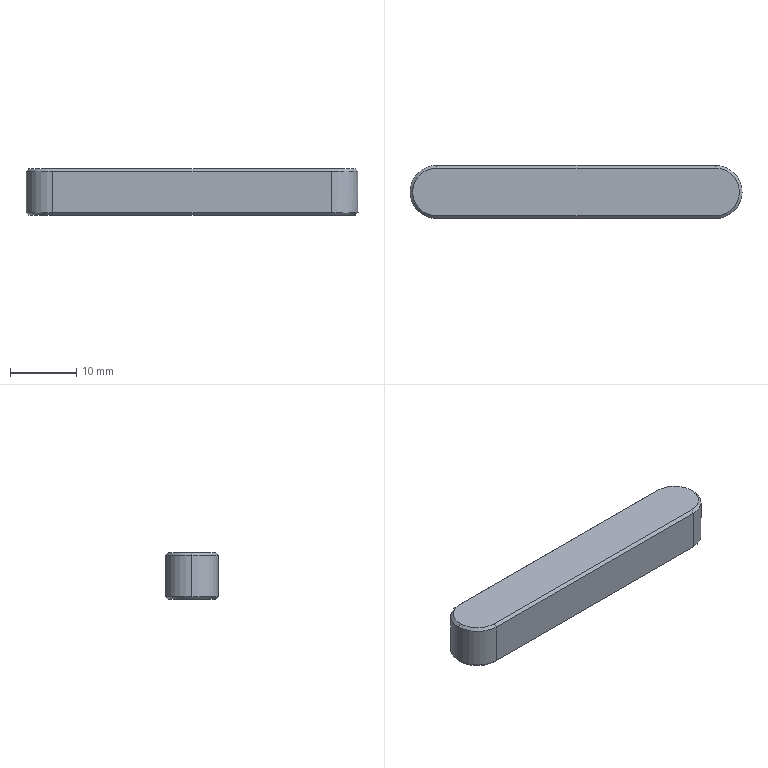Part | STEP file | plain parallel_keys_GB_CONNECTING_PIECE_KEYS_CSK 8X50 | 1 solid | 17 faces | box 50 x 8 x 7 mm | volume 2687 mm3 | plane 8 | cone 6 | cylinder 3 | commonest cylinder face diameters 8 x3
STEP:
#1=CARTESIAN_POINT('',(0.,0.,0.));
#2=DIRECTION('',(0.,0.,1.));
#3=DIRECTION('',(1.,0.,0.));
#4=AXIS2_PLACEMENT_3D('',#1,#2,#3);
#5=CARTESIAN_POINT('',(3.6,0.,-3.5));
#6=VERTEX_POINT('',#5);
#7=CARTESIAN_POINT('',(0.,-3.6,-3.5));
#8=VERTEX_POINT('',#7);
#9=CARTESIAN_POINT('',(0.,0.,-3.5));
#10=DIRECTION('',(0.,0.,-1.));
#11=DIRECTION('',(1.,0.,0.));
#12=AXIS2_PLACEMENT_3D('',#9,#10,#11);
#13=CIRCLE('',#12,3.6);
#14=CARTESIAN_POINT('',(0.,0.,-3.1));
#15=DIRECTION('',(0.,0.,1.));
#16=DIRECTION('',(1.,0.,0.));
#17=AXIS2_PLACEMENT_3D('',#14,#15,#16);
#18=CONICAL_SURFACE('',#17,4.,0.7854);
#19=CARTESIAN_POINT('',(6.283,-0.4));
#20=DIRECTION('',(-1.,0.));
#21=VECTOR('',#20,1.);
#22=LINE('',#19,#21);
#23=(GEOMETRIC_REPRESENTATION_CONTEXT(2)PARAMETRIC_REPRESENTATION_CONTEXT()REPRESENTATION_CONTEXT('',''));
#24=DEFINITIONAL_REPRESENTATION('',(#22),#23);
#25=PCURVE('',#18,#24);
#26=CARTESIAN_POINT('',(-42.,0.,-3.5));
#27=DIRECTION('',(0.,0.,-1.));
#28=DIRECTION('',(-1.,0.,0.));
#29=AXIS2_PLACEMENT_3D('',#26,#27,#28);
#30=PLANE('',#29);
#31=CARTESIAN_POINT('',(-42.,0.));
#32=DIRECTION('',(-1.,0.));
#33=AXIS2_PLACEMENT_2D('',#31,#32);
#34=CIRCLE('',#33,3.6);
#35=(GEOMETRIC_REPRESENTATION_CONTEXT(2)PARAMETRIC_REPRESENTATION_CONTEXT()REPRESENTATION_CONTEXT('',''));
#36=DEFINITIONAL_REPRESENTATION('',(#34),#35);
#37=PCURVE('',#30,#36);
#38=SURFACE_CURVE('',#13,(#25,#37),.PCURVE_S1.);
#39=EDGE_CURVE('',#6,#8,#38,.T.);
#40=ORIENTED_EDGE('',*,*,#39,.F.);
#41=CARTESIAN_POINT('',(4.,0.,-3.1));
#42=VERTEX_POINT('',#41);
#43=CARTESIAN_POINT('',(4.,0.,-3.1));
#44=DIRECTION('',(0.7071,0.,0.7071));
#45=VECTOR('',#44,1.);
#46=LINE('',#43,#45);
#47=CARTESIAN_POINT('',(6.283,0.));
#48=DIRECTION('',(0.,1.));
#49=VECTOR('',#48,1.);
#50=LINE('',#47,#49);
#51=(GEOMETRIC_REPRESENTATION_CONTEXT(2)PARAMETRIC_REPRESENTATION_CONTEXT()REPRESENTATION_CONTEXT('',''));
#52=DEFINITIONAL_REPRESENTATION('',(#50),#51);
#53=PCURVE('',#18,#52);
#54=CARTESIAN_POINT('',(0.,0.,-3.1));
#55=DIRECTION('',(0.,0.,1.));
#56=DIRECTION('',(1.,0.,0.));
#57=AXIS2_PLACEMENT_3D('',#54,#55,#56);
#58=CONICAL_SURFACE('',#57,4.,0.7854);
#59=CARTESIAN_POINT('',(0.,0.));
#60=DIRECTION('',(0.,1.));
#61=VECTOR('',#60,1.);
#62=LINE('',#59,#61);
#63=(GEOMETRIC_REPRESENTATION_CONTEXT(2)PARAMETRIC_REPRESENTATION_CONTEXT()REPRESENTATION_CONTEXT('',''));
#64=DEFINITIONAL_REPRESENTATION('',(#62),#63);
#65=PCURVE('',#58,#64);
#66=SURFACE_CURVE('',#46,(#53,#65),.PCURVE_S1.);
#67=EDGE_CURVE('',#6,#42,#66,.T.);
#68=ORIENTED_EDGE('',*,*,#67,.T.);
#69=CARTESIAN_POINT('',(0.,-4.,-3.1));
#70=VERTEX_POINT('',#69);
#71=CARTESIAN_POINT('',(0.,0.,-3.1));
#72=DIRECTION('',(0.,0.,-1.));
#73=DIRECTION('',(1.,0.,0.));
#74=AXIS2_PLACEMENT_3D('',#71,#72,#73);
#75=CIRCLE('',#74,4.);
#76=CARTESIAN_POINT('',(6.283,0.));
#77=DIRECTION('',(-1.,0.));
#78=VECTOR('',#77,1.);
#79=LINE('',#76,#78);
#80=(GEOMETRIC_REPRESENTATION_CONTEXT(2)PARAMETRIC_REPRESENTATION_CONTEXT()REPRESENTATION_CONTEXT('',''));
#81=DEFINITIONAL_REPRESENTATION('',(#79),#80);
#82=PCURVE('',#18,#81);
#83=CARTESIAN_POINT('',(0.,0.,3.5));
#84=DIRECTION('',(0.,0.,-1.));
#85=DIRECTION('',(-1.,0.,0.));
#86=AXIS2_PLACEMENT_3D('',#83,#84,#85);
#87=CYLINDRICAL_SURFACE('',#86,4.);
#88=CARTESIAN_POINT('',(3.142,6.6));
#89=DIRECTION('',(1.,0.));
#90=VECTOR('',#89,1.);
#91=LINE('',#88,#90);
#92=(GEOMETRIC_REPRESENTATION_CONTEXT(2)PARAMETRIC_REPRESENTATION_CONTEXT()REPRESENTATION_CONTEXT('',''));
#93=DEFINITIONAL_REPRESENTATION('',(#91),#92);
#94=PCURVE('',#87,#93);
#95=SURFACE_CURVE('',#75,(#82,#94),.PCURVE_S1.);
#96=EDGE_CURVE('',#42,#70,#95,.T.);
#97=ORIENTED_EDGE('',*,*,#96,.T.);
#98=CARTESIAN_POINT('',(0.,-4.,-3.1));
#99=DIRECTION('',(0.,-0.7071,0.7071));
#100=VECTOR('',#99,1.);
#101=LINE('',#98,#100);
#102=CARTESIAN_POINT('',(4.712,0.));
#103=DIRECTION('',(0.,1.));
#104=VECTOR('',#103,1.);
#105=LINE('',#102,#104);
#106=(GEOMETRIC_REPRESENTATION_CONTEXT(2)PARAMETRIC_REPRESENTATION_CONTEXT()REPRESENTATION_CONTEXT('',''));
#107=DEFINITIONAL_REPRESENTATION('',(#105),#106);
#108=PCURVE('',#18,#107);
#109=CARTESIAN_POINT('',(0.,-4.,-3.1));
#110=DIRECTION('',(0.,-0.7071,-0.7071));
#111=DIRECTION('',(0.,0.7071,-0.7071));
#112=AXIS2_PLACEMENT_3D('',#109,#110,#111);
#113=PLANE('',#112);
#114=CARTESIAN_POINT('',(0.,0.));
#115=DIRECTION('',(-1.,0.));
#116=VECTOR('',#115,1.);
#117=LINE('',#114,#116);
#118=(GEOMETRIC_REPRESENTATION_CONTEXT(2)PARAMETRIC_REPRESENTATION_CONTEXT()REPRESENTATION_CONTEXT('',''));
#119=DEFINITIONAL_REPRESENTATION('',(#117),#118);
#120=PCURVE('',#113,#119);
#121=SURFACE_CURVE('',#101,(#108,#120),.PCURVE_S1.);
#122=EDGE_CURVE('',#8,#70,#121,.T.);
#123=ORIENTED_EDGE('',*,*,#122,.F.);
#124=EDGE_LOOP('',(#40,#68,#97,#123));
#125=FACE_BOUND('',#124,.T.);
#126=ADVANCED_FACE('',(#125),#18,.T.);
#127=CARTESIAN_POINT('',(-42.,-4.,3.1));
#128=VERTEX_POINT('',#127);
#129=CARTESIAN_POINT('',(-46.,0.,3.1));
#130=VERTEX_POINT('',#129);
#131=CARTESIAN_POINT('',(-42.,0.,3.1));
#132=DIRECTION('',(0.,0.,-1.));
#133=DIRECTION('',(-1.,0.,0.));
#134=AXIS2_PLACEMENT_3D('',#131,#132,#133);
#135=CIRCLE('',#134,4.);
#136=CARTESIAN_POINT('',(-42.,0.,3.5));
#137=DIRECTION('',(0.,0.,-1.));
#138=DIRECTION('',(-1.,0.,0.));
#139=AXIS2_PLACEMENT_3D('',#136,#137,#138);
#140=CYLINDRICAL_SURFACE('',#139,4.);
#141=CARTESIAN_POINT('',(0.,0.4));
#142=DIRECTION('',(1.,0.));
#143=VECTOR('',#142,1.);
#144=LINE('',#141,#143);
#145=(GEOMETRIC_REPRESENTATION_CONTEXT(2)PARAMETRIC_REPRESENTATION_CONTEXT()REPRESENTATION_CONTEXT('',''));
#146=DEFINITIONAL_REPRESENTATION('',(#144),#145);
#147=PCURVE('',#140,#146);
#148=CARTESIAN_POINT('',(-42.,0.,3.1));
#149=DIRECTION('',(0.,0.,-1.));
#150=DIRECTION('',(-1.,0.,0.));
#151=AXIS2_PLACEMENT_3D('',#148,#149,#150);
#152=CONICAL_SURFACE('',#151,4.,0.7854);
#153=CARTESIAN_POINT('',(0.,0.));
#154=DIRECTION('',(1.,0.));
#155=VECTOR('',#154,1.);
#156=LINE('',#153,#155);
#157=(GEOMETRIC_REPRESENTATION_CONTEXT(2)PARAMETRIC_REPRESENTATION_CONTEXT()REPRESENTATION_CONTEXT('',''));
#158=DEFINITIONAL_REPRESENTATION('',(#156),#157);
#159=PCURVE('',#152,#158);
#160=SURFACE_CURVE('',#135,(#147,#159),.PCURVE_S1.);
#161=EDGE_CURVE('',#128,#130,#160,.T.);
#162=ORIENTED_EDGE('',*,*,#161,.T.);
#163=CARTESIAN_POINT('',(-46.,0.,-3.1));
#164=VERTEX_POINT('',#163);
#165=CARTESIAN_POINT('',(-46.,0.,3.5));
#166=DIRECTION('',(0.,0.,-1.));
#167=VECTOR('',#166,1.);
#168=LINE('',#165,#167);
#169=CARTESIAN_POINT('',(6.283,0.));
#170=DIRECTION('',(0.,1.));
#171=VECTOR('',#170,1.);
#172=LINE('',#169,#171);
#173=(GEOMETRIC_REPRESENTATION_CONTEXT(2)PARAMETRIC_REPRESENTATION_CONTEXT()REPRESENTATION_CONTEXT('',''));
#174=DEFINITIONAL_REPRESENTATION('',(#172),#173);
#175=PCURVE('',#140,#174);
#176=CARTESIAN_POINT('',(-42.,0.,3.5));
#177=DIRECTION('',(0.,0.,-1.));
#178=DIRECTION('',(-1.,0.,0.));
#179=AXIS2_PLACEMENT_3D('',#176,#177,#178);
#180=CYLINDRICAL_SURFACE('',#179,4.);
#181=CARTESIAN_POINT('',(0.,0.));
#182=DIRECTION('',(0.,1.));
#183=VECTOR('',#182,1.);
#184=LINE('',#181,#183);
#185=(GEOMETRIC_REPRESENTATION_CONTEXT(2)PARAMETRIC_REPRESENTATION_CONTEXT()REPRESENTATION_CONTEXT('',''));
#186=DEFINITIONAL_REPRESENTATION('',(#184),#185);
#187=PCURVE('',#180,#186);
#188=SURFACE_CURVE('',#168,(#175,#187),.PCURVE_S1.);
#189=EDGE_CURVE('',#130,#164,#188,.T.);
#190=ORIENTED_EDGE('',*,*,#189,.T.);
#191=CARTESIAN_POINT('',(-42.,-4.,-3.1));
#192=VERTEX_POINT('',#191);
#193=CARTESIAN_POINT('',(-42.,0.,-3.1));
#194=DIRECTION('',(0.,0.,-1.));
#195=DIRECTION('',(1.,0.,0.));
#196=AXIS2_PLACEMENT_3D('',#193,#194,#195);
#197=CIRCLE('',#196,4.);
#198=CARTESIAN_POINT('',(3.142,6.6));
#199=DIRECTION('',(1.,0.));
#200=VECTOR('',#199,1.);
#201=LINE('',#198,#200);
#202=(GEOMETRIC_REPRESENTATION_CONTEXT(2)PARAMETRIC_REPRESENTATION_CONTEXT()REPRESENTATION_CONTEXT('',''));
#203=DEFINITIONAL_REPRESENTATION('',(#201),#202);
#204=PCURVE('',#140,#203);
#205=CARTESIAN_POINT('',(-42.,0.,-3.1));
#206=DIRECTION('',(0.,0.,1.));
#207=DIRECTION('',(1.,0.,0.));
#208=AXIS2_PLACEMENT_3D('',#205,#206,#207);
#209=CONICAL_SURFACE('',#208,4.,0.7854);
#210=CARTESIAN_POINT('',(6.283,0.));
#211=DIRECTION('',(-1.,0.));
#212=VECTOR('',#211,1.);
#213=LINE('',#210,#212);
#214=(GEOMETRIC_REPRESENTATION_CONTEXT(2)PARAMETRIC_REPRESENTATION_CONTEXT()REPRESENTATION_CONTEXT('',''));
#215=DEFINITIONAL_REPRESENTATION('',(#213),#214);
#216=PCURVE('',#209,#215);
#217=SURFACE_CURVE('',#197,(#204,#216),.PCURVE_S1.);
#218=EDGE_CURVE('',#192,#164,#217,.T.);
#219=ORIENTED_EDGE('',*,*,#218,.F.);
#220=CARTESIAN_POINT('',(-42.,-4.,3.5));
#221=DIRECTION('',(0.,0.,1.));
#222=VECTOR('',#221,1.);
#223=LINE('',#220,#222);
#224=CARTESIAN_POINT('',(4.712,0.));
#225=DIRECTION('',(0.,-1.));
#226=VECTOR('',#225,1.);
#227=LINE('',#224,#226);
#228=(GEOMETRIC_REPRESENTATION_CONTEXT(2)PARAMETRIC_REPRESENTATION_CONTEXT()REPRESENTATION_CONTEXT('',''));
#229=DEFINITIONAL_REPRESENTATION('',(#227),#228);
#230=PCURVE('',#140,#229);
#231=CARTESIAN_POINT('',(0.,-4.,3.5));
#232=DIRECTION('',(0.,1.,0.));
#233=DIRECTION('',(-1.,0.,0.));
#234=AXIS2_PLACEMENT_3D('',#231,#232,#233);
#235=PLANE('',#234);
#236=CARTESIAN_POINT('',(42.,0.));
#237=DIRECTION('',(0.,1.));
#238=VECTOR('',#237,1.);
#239=LINE('',#236,#238);
#240=(GEOMETRIC_REPRESENTATION_CONTEXT(2)PARAMETRIC_REPRESENTATION_CONTEXT()REPRESENTATION_CONTEXT('',''));
#241=DEFINITIONAL_REPRESENTATION('',(#239),#240);
#242=PCURVE('',#235,#241);
#243=SURFACE_CURVE('',#223,(#230,#242),.PCURVE_S1.);
#244=EDGE_CURVE('',#192,#128,#243,.T.);
#245=ORIENTED_EDGE('',*,*,#244,.T.);
#246=EDGE_LOOP('',(#162,#190,#219,#245));
#247=FACE_BOUND('',#246,.T.);
#248=ADVANCED_FACE('',(#247),#140,.T.);
#249=CARTESIAN_POINT('',(-42.,-3.6,3.5));
#250=VERTEX_POINT('',#249);
#251=CARTESIAN_POINT('',(-45.6,0.,3.5));
#252=VERTEX_POINT('',#251);
#253=CARTESIAN_POINT('',(-42.,0.,3.5));
#254=DIRECTION('',(0.,0.,-1.));
#255=DIRECTION('',(-1.,0.,0.));
#256=AXIS2_PLACEMENT_3D('',#253,#254,#255);
#257=CIRCLE('',#256,3.6);
#258=CARTESIAN_POINT('',(0.,-0.4));
#259=DIRECTION('',(1.,0.));
#260=VECTOR('',#259,1.);
#261=LINE('',#258,#260);
#262=(GEOMETRIC_REPRESENTATION_CONTEXT(2)PARAMETRIC_REPRESENTATION_CONTEXT()REPRESENTATION_CONTEXT('',''));
#263=DEFINITIONAL_REPRESENTATION('',(#261),#262);
#264=PCURVE('',#152,#263);
#265=CARTESIAN_POINT('',(-42.,0.,3.5));
#266=DIRECTION('',(0.,0.,-1.));
#267=DIRECTION('',(-1.,0.,0.));
#268=AXIS2_PLACEMENT_3D('',#265,#266,#267);
#269=PLANE('',#268);
#270=CARTESIAN_POINT('',(0.,0.));
#271=DIRECTION('',(1.,0.));
#272=AXIS2_PLACEMENT_2D('',#270,#271);
#273=CIRCLE('',#272,3.6);
#274=(GEOMETRIC_REPRESENTATION_CONTEXT(2)PARAMETRIC_REPRESENTATION_CONTEXT()REPRESENTATION_CONTEXT('',''));
#275=DEFINITIONAL_REPRESENTATION('',(#273),#274);
#276=PCURVE('',#269,#275);
#277=SURFACE_CURVE('',#257,(#264,#276),.PCURVE_S1.);
#278=EDGE_CURVE('',#250,#252,#277,.T.);
#279=ORIENTED_EDGE('',*,*,#278,.T.);
#280=CARTESIAN_POINT('',(-46.,0.,3.1));
#281=DIRECTION('',(-0.7071,0.,-0.7071));
#282=VECTOR('',#281,1.);
#283=LINE('',#280,#282);
#284=CARTESIAN_POINT('',(6.283,0.));
#285=DIRECTION('',(0.,1.));
#286=VECTOR('',#285,1.);
#287=LINE('',#284,#286);
#288=(GEOMETRIC_REPRESENTATION_CONTEXT(2)PARAMETRIC_REPRESENTATION_CONTEXT()REPRESENTATION_CONTEXT('',''));
#289=DEFINITIONAL_REPRESENTATION('',(#287),#288);
#290=PCURVE('',#152,#289);
#291=CARTESIAN_POINT('',(-42.,0.,3.1));
#292=DIRECTION('',(0.,0.,-1.));
#293=DIRECTION('',(-1.,0.,0.));
#294=AXIS2_PLACEMENT_3D('',#291,#292,#293);
#295=CONICAL_SURFACE('',#294,4.,0.7854);
#296=CARTESIAN_POINT('',(0.,0.));
#297=DIRECTION('',(0.,1.));
#298=VECTOR('',#297,1.);
#299=LINE('',#296,#298);
#300=(GEOMETRIC_REPRESENTATION_CONTEXT(2)PARAMETRIC_REPRESENTATION_CONTEXT()REPRESENTATION_CONTEXT('',''));
#301=DEFINITIONAL_REPRESENTATION('',(#299),#300);
#302=PCURVE('',#295,#301);
#303=SURFACE_CURVE('',#283,(#290,#302),.PCURVE_S1.);
#304=EDGE_CURVE('',#252,#130,#303,.T.);
#305=ORIENTED_EDGE('',*,*,#304,.T.);
#306=ORIENTED_EDGE('',*,*,#161,.F.);
#307=CARTESIAN_POINT('',(-42.,-498958.,-498950.9));
#308=DIRECTION('',(0.,0.7071,0.7071));
#309=VECTOR('',#308,1.);
#310=LINE('',#307,#309);
#311=CARTESIAN_POINT('',(4.712,498954.));
#312=DIRECTION('',(0.,-1.));
#313=VECTOR('',#312,1.);
#314=LINE('',#311,#313);
#315=(GEOMETRIC_REPRESENTATION_CONTEXT(2)PARAMETRIC_REPRESENTATION_CONTEXT()REPRESENTATION_CONTEXT('',''));
#316=DEFINITIONAL_REPRESENTATION('',(#314),#315);
#317=PCURVE('',#152,#316);
#318=CARTESIAN_POINT('',(-42.,-3.6,3.5));
#319=DIRECTION('',(0.,0.7071,-0.7071));
#320=DIRECTION('',(0.,0.7071,0.7071));
#321=AXIS2_PLACEMENT_3D('',#318,#319,#320);
#322=PLANE('',#321);
#323=CARTESIAN_POINT('',(-705628.079,0.));
#324=DIRECTION('',(1.,0.));
#325=VECTOR('',#324,1.);
#326=LINE('',#323,#325);
#327=(GEOMETRIC_REPRESENTATION_CONTEXT(2)PARAMETRIC_REPRESENTATION_CONTEXT()REPRESENTATION_CONTEXT('',''));
#328=DEFINITIONAL_REPRESENTATION('',(#326),#327);
#329=PCURVE('',#322,#328);
#330=SURFACE_CURVE('',#310,(#317,#329),.PCURVE_S1.);
#331=EDGE_CURVE('',#128,#250,#330,.T.);
#332=ORIENTED_EDGE('',*,*,#331,.T.);
#333=EDGE_LOOP('',(#279,#305,#306,#332));
#334=FACE_BOUND('',#333,.T.);
#335=ADVANCED_FACE('',(#334),#152,.T.);
#336=CARTESIAN_POINT('',(-42.,-3.6,-3.5));
#337=VERTEX_POINT('',#336);
#338=CARTESIAN_POINT('',(-42.,3.6,-3.5));
#339=VERTEX_POINT('',#338);
#340=CARTESIAN_POINT('',(-42.,0.,-3.5));
#341=DIRECTION('',(0.,0.,-1.));
#342=DIRECTION('',(1.,0.,0.));
#343=AXIS2_PLACEMENT_3D('',#340,#341,#342);
#344=CIRCLE('',#343,3.6);
#345=CARTESIAN_POINT('',(0.,0.));
#346=DIRECTION('',(-1.,0.));
#347=AXIS2_PLACEMENT_2D('',#345,#346);
#348=CIRCLE('',#347,3.6);
#349=(GEOMETRIC_REPRESENTATION_CONTEXT(2)PARAMETRIC_REPRESENTATION_CONTEXT()REPRESENTATION_CONTEXT('',''));
#350=DEFINITIONAL_REPRESENTATION('',(#348),#349);
#351=PCURVE('',#30,#350);
#352=CARTESIAN_POINT('',(6.283,-0.4));
#353=DIRECTION('',(-1.,0.));
#354=VECTOR('',#353,1.);
#355=LINE('',#352,#354);
#356=(GEOMETRIC_REPRESENTATION_CONTEXT(2)PARAMETRIC_REPRESENTATION_CONTEXT()REPRESENTATION_CONTEXT('',''));
#357=DEFINITIONAL_REPRESENTATION('',(#355),#356);
#358=PCURVE('',#209,#357);
#359=SURFACE_CURVE('',#344,(#351,#358),.PCURVE_S1.);
#360=EDGE_CURVE('',#337,#339,#359,.T.);
#361=ORIENTED_EDGE('',*,*,#360,.T.);
#362=CARTESIAN_POINT('',(0.,3.6,-3.5));
#363=VERTEX_POINT('',#362);
#364=CARTESIAN_POINT('',(-42.,3.6,-3.5));
#365=DIRECTION('',(1.,0.,0.));
#366=VECTOR('',#365,1.);
#367=LINE('',#364,#366);
#368=CARTESIAN_POINT('',(0.,3.6));
#369=DIRECTION('',(-1.,0.));
#370=VECTOR('',#369,1.);
#371=LINE('',#368,#370);
#372=(GEOMETRIC_REPRESENTATION_CONTEXT(2)PARAMETRIC_REPRESENTATION_CONTEXT()REPRESENTATION_CONTEXT('',''));
#373=DEFINITIONAL_REPRESENTATION('',(#371),#372);
#374=PCURVE('',#30,#373);
#375=CARTESIAN_POINT('',(-42.,4.,-3.1));
#376=DIRECTION('',(0.,0.7071,-0.7071));
#377=DIRECTION('',(0.,0.7071,0.7071));
#378=AXIS2_PLACEMENT_3D('',#375,#376,#377);
#379=PLANE('',#378);
#380=CARTESIAN_POINT('',(-0.5657,0.));
#381=DIRECTION('',(0.,1.));
#382=VECTOR('',#381,1.);
#383=LINE('',#380,#382);
#384=(GEOMETRIC_REPRESENTATION_CONTEXT(2)PARAMETRIC_REPRESENTATION_CONTEXT()REPRESENTATION_CONTEXT('',''));
#385=DEFINITIONAL_REPRESENTATION('',(#383),#384);
#386=PCURVE('',#379,#385);
#387=SURFACE_CURVE('',#367,(#374,#386),.PCURVE_S1.);
#388=EDGE_CURVE('',#339,#363,#387,.T.);
#389=ORIENTED_EDGE('',*,*,#388,.T.);
#390=CARTESIAN_POINT('',(0.,0.,-3.5));
#391=DIRECTION('',(0.,0.,-1.));
#392=DIRECTION('',(1.,0.,0.));
#393=AXIS2_PLACEMENT_3D('',#390,#391,#392);
#394=CIRCLE('',#393,3.6);
#395=CARTESIAN_POINT('',(-42.,0.));
#396=DIRECTION('',(-1.,0.));
#397=AXIS2_PLACEMENT_2D('',#395,#396);
#398=CIRCLE('',#397,3.6);
#399=(GEOMETRIC_REPRESENTATION_CONTEXT(2)PARAMETRIC_REPRESENTATION_CONTEXT()REPRESENTATION_CONTEXT('',''));
#400=DEFINITIONAL_REPRESENTATION('',(#398),#399);
#401=PCURVE('',#30,#400);
#402=CARTESIAN_POINT('',(6.283,-0.4));
#403=DIRECTION('',(-1.,0.));
#404=VECTOR('',#403,1.);
#405=LINE('',#402,#404);
#406=(GEOMETRIC_REPRESENTATION_CONTEXT(2)PARAMETRIC_REPRESENTATION_CONTEXT()REPRESENTATION_CONTEXT('',''));
#407=DEFINITIONAL_REPRESENTATION('',(#405),#406);
#408=PCURVE('',#58,#407);
#409=SURFACE_CURVE('',#394,(#401,#408),.PCURVE_S1.);
#410=EDGE_CURVE('',#363,#6,#409,.T.);
#411=ORIENTED_EDGE('',*,*,#410,.T.);
#412=ORIENTED_EDGE('',*,*,#39,.T.);
#413=CARTESIAN_POINT('',(-42.,-3.6,-3.5));
#414=DIRECTION('',(-1.,0.,0.));
#415=VECTOR('',#414,1.);
#416=LINE('',#413,#415);
#417=CARTESIAN_POINT('',(0.,-3.6));
#418=DIRECTION('',(1.,0.));
#419=VECTOR('',#418,1.);
#420=LINE('',#417,#419);
#421=(GEOMETRIC_REPRESENTATION_CONTEXT(2)PARAMETRIC_REPRESENTATION_CONTEXT()REPRESENTATION_CONTEXT('',''));
#422=DEFINITIONAL_REPRESENTATION('',(#420),#421);
#423=PCURVE('',#30,#422);
#424=CARTESIAN_POINT('',(0.5657,-42.));
#425=DIRECTION('',(0.,-1.));
#426=VECTOR('',#425,1.);
#427=LINE('',#424,#426);
#428=(GEOMETRIC_REPRESENTATION_CONTEXT(2)PARAMETRIC_REPRESENTATION_CONTEXT()REPRESENTATION_CONTEXT('',''));
#429=DEFINITIONAL_REPRESENTATION('',(#427),#428);
#430=PCURVE('',#113,#429);
#431=SURFACE_CURVE('',#416,(#423,#430),.PCURVE_S1.);
#432=EDGE_CURVE('',#8,#337,#431,.T.);
#433=ORIENTED_EDGE('',*,*,#432,.T.);
#434=EDGE_LOOP('',(#361,#389,#411,#412,#433));
#435=FACE_BOUND('',#434,.T.);
#436=ADVANCED_FACE('',(#435),#30,.T.);
#437=CARTESIAN_POINT('',(-42.,4.,-3.1));
#438=VERTEX_POINT('',#437);
#439=CARTESIAN_POINT('',(-42.,4.,-3.1));
#440=DIRECTION('',(0.,0.7071,0.7071));
#441=VECTOR('',#440,1.);
#442=LINE('',#439,#441);
#443=CARTESIAN_POINT('',(0.,0.));
#444=DIRECTION('',(1.,0.));
#445=VECTOR('',#444,1.);
#446=LINE('',#443,#445);
#447=(GEOMETRIC_REPRESENTATION_CONTEXT(2)PARAMETRIC_REPRESENTATION_CONTEXT()REPRESENTATION_CONTEXT('',''));
#448=DEFINITIONAL_REPRESENTATION('',(#446),#447);
#449=PCURVE('',#379,#448);
#450=CARTESIAN_POINT('',(1.571,0.));
#451=DIRECTION('',(0.,1.));
#452=VECTOR('',#451,1.);
#453=LINE('',#450,#452);
#454=(GEOMETRIC_REPRESENTATION_CONTEXT(2)PARAMETRIC_REPRESENTATION_CONTEXT()REPRESENTATION_CONTEXT('',''));
#455=DEFINITIONAL_REPRESENTATION('',(#453),#454);
#456=PCURVE('',#209,#455);
#457=SURFACE_CURVE('',#442,(#449,#456),.PCURVE_S1.);
#458=EDGE_CURVE('',#339,#438,#457,.T.);
#459=ORIENTED_EDGE('',*,*,#458,.T.);
#460=CARTESIAN_POINT('',(0.,4.,-3.1));
#461=VERTEX_POINT('',#460);
#462=CARTESIAN_POINT('',(-42.,4.,-3.1));
#463=DIRECTION('',(1.,0.,0.));
#464=VECTOR('',#463,1.);
#465=LINE('',#462,#464);
#466=CARTESIAN_POINT('',(0.,0.));
#467=DIRECTION('',(0.,1.));
#468=VECTOR('',#467,1.);
#469=LINE('',#466,#468);
#470=(GEOMETRIC_REPRESENTATION_CONTEXT(2)PARAMETRIC_REPRESENTATION_CONTEXT()REPRESENTATION_CONTEXT('',''));
#471=DEFINITIONAL_REPRESENTATION('',(#469),#470);
#472=PCURVE('',#379,#471);
#473=CARTESIAN_POINT('',(-42.,4.,3.5));
#474=DIRECTION('',(0.,-1.,0.));
#475=DIRECTION('',(1.,0.,0.));
#476=AXIS2_PLACEMENT_3D('',#473,#474,#475);
#477=PLANE('',#476);
#478=CARTESIAN_POINT('',(0.,-6.6));
#479=DIRECTION('',(1.,0.));
#480=VECTOR('',#479,1.);
#481=LINE('',#478,#480);
#482=(GEOMETRIC_REPRESENTATION_CONTEXT(2)PARAMETRIC_REPRESENTATION_CONTEXT()REPRESENTATION_CONTEXT('',''));
#483=DEFINITIONAL_REPRESENTATION('',(#481),#482);
#484=PCURVE('',#477,#483);
#485=SURFACE_CURVE('',#465,(#472,#484),.PCURVE_S1.);
#486=EDGE_CURVE('',#438,#461,#485,.T.);
#487=ORIENTED_EDGE('',*,*,#486,.T.);
#488=CARTESIAN_POINT('',(0.,4.,-3.1));
#489=DIRECTION('',(0.,-0.7071,-0.7071));
#490=VECTOR('',#489,1.);
#491=LINE('',#488,#490);
#492=CARTESIAN_POINT('',(0.,42.));
#493=DIRECTION('',(-1.,0.));
#494=VECTOR('',#493,1.);
#495=LINE('',#492,#494);
#496=(GEOMETRIC_REPRESENTATION_CONTEXT(2)PARAMETRIC_REPRESENTATION_CONTEXT()REPRESENTATION_CONTEXT('',''));
#497=DEFINITIONAL_REPRESENTATION('',(#495),#496);
#498=PCURVE('',#379,#497);
#499=CARTESIAN_POINT('',(1.571,0.));
#500=DIRECTION('',(0.,-1.));
#501=VECTOR('',#500,1.);
#502=LINE('',#499,#501);
#503=(GEOMETRIC_REPRESENTATION_CONTEXT(2)PARAMETRIC_REPRESENTATION_CONTEXT()REPRESENTATION_CONTEXT('',''));
#504=DEFINITIONAL_REPRESENTATION('',(#502),#503);
#505=PCURVE('',#58,#504);
#506=SURFACE_CURVE('',#491,(#498,#505),.PCURVE_S1.);
#507=EDGE_CURVE('',#461,#363,#506,.T.);
#508=ORIENTED_EDGE('',*,*,#507,.T.);
#509=ORIENTED_EDGE('',*,*,#388,.F.);
#510=EDGE_LOOP('',(#459,#487,#508,#509));
#511=FACE_BOUND('',#510,.T.);
#512=ADVANCED_FACE('',(#511),#379,.T.);
#513=CARTESIAN_POINT('',(-42.,-499007.1,499000.));
#514=DIRECTION('',(0.,-0.7071,0.7071));
#515=VECTOR('',#514,1.);
#516=LINE('',#513,#515);
#517=CARTESIAN_POINT('',(4.712,499003.1));
#518=DIRECTION('',(0.,1.));
#519=VECTOR('',#518,1.);
#520=LINE('',#517,#519);
#521=(GEOMETRIC_REPRESENTATION_CONTEXT(2)PARAMETRIC_REPRESENTATION_CONTEXT()REPRESENTATION_CONTEXT('',''));
#522=DEFINITIONAL_REPRESENTATION('',(#520),#521);
#523=PCURVE('',#209,#522);
#524=CARTESIAN_POINT('',(-705696.952,-42.));
#525=DIRECTION('',(-1.,0.));
#526=VECTOR('',#525,1.);
#527=LINE('',#524,#526);
#528=(GEOMETRIC_REPRESENTATION_CONTEXT(2)PARAMETRIC_REPRESENTATION_CONTEXT()REPRESENTATION_CONTEXT('',''));
#529=DEFINITIONAL_REPRESENTATION('',(#527),#528);
#530=PCURVE('',#113,#529);
#531=SURFACE_CURVE('',#516,(#523,#530),.PCURVE_S1.);
#532=EDGE_CURVE('',#337,#192,#531,.T.);
#533=ORIENTED_EDGE('',*,*,#532,.T.);
#534=ORIENTED_EDGE('',*,*,#218,.T.);
#535=CARTESIAN_POINT('',(-42.,0.,-3.1));
#536=DIRECTION('',(0.,0.,-1.));
#537=DIRECTION('',(1.,0.,0.));
#538=AXIS2_PLACEMENT_3D('',#535,#536,#537);
#539=CIRCLE('',#538,4.);
#540=CARTESIAN_POINT('',(6.283,0.));
#541=DIRECTION('',(-1.,0.));
#542=VECTOR('',#541,1.);
#543=LINE('',#540,#542);
#544=(GEOMETRIC_REPRESENTATION_CONTEXT(2)PARAMETRIC_REPRESENTATION_CONTEXT()REPRESENTATION_CONTEXT('',''));
#545=DEFINITIONAL_REPRESENTATION('',(#543),#544);
#546=PCURVE('',#209,#545);
#547=CARTESIAN_POINT('',(-3.142,6.6));
#548=DIRECTION('',(1.,0.));
#549=VECTOR('',#548,1.);
#550=LINE('',#547,#549);
#551=(GEOMETRIC_REPRESENTATION_CONTEXT(2)PARAMETRIC_REPRESENTATION_CONTEXT()REPRESENTATION_CONTEXT('',''));
#552=DEFINITIONAL_REPRESENTATION('',(#550),#551);
#553=PCURVE('',#180,#552);
#554=SURFACE_CURVE('',#539,(#546,#553),.PCURVE_S1.);
#555=EDGE_CURVE('',#164,#438,#554,.T.);
#556=ORIENTED_EDGE('',*,*,#555,.T.);
#557=ORIENTED_EDGE('',*,*,#458,.F.);
#558=ORIENTED_EDGE('',*,*,#360,.F.);
#559=EDGE_LOOP('',(#533,#534,#556,#557,#558));
#560=FACE_BOUND('',#559,.T.);
#561=ADVANCED_FACE('',(#560),#209,.T.);
#562=ORIENTED_EDGE('',*,*,#122,.T.);
#563=CARTESIAN_POINT('',(0.,-4.,-3.1));
#564=DIRECTION('',(-1.,0.,0.));
#565=VECTOR('',#564,1.);
#566=LINE('',#563,#565);
#567=CARTESIAN_POINT('',(0.,0.));
#568=DIRECTION('',(0.,-1.));
#569=VECTOR('',#568,1.);
#570=LINE('',#567,#569);
#571=(GEOMETRIC_REPRESENTATION_CONTEXT(2)PARAMETRIC_REPRESENTATION_CONTEXT()REPRESENTATION_CONTEXT('',''));
#572=DEFINITIONAL_REPRESENTATION('',(#570),#571);
#573=PCURVE('',#113,#572);
#574=CARTESIAN_POINT('',(0.,-6.6));
#575=DIRECTION('',(1.,0.));
#576=VECTOR('',#575,1.);
#577=LINE('',#574,#576);
#578=(GEOMETRIC_REPRESENTATION_CONTEXT(2)PARAMETRIC_REPRESENTATION_CONTEXT()REPRESENTATION_CONTEXT('',''));
#579=DEFINITIONAL_REPRESENTATION('',(#577),#578);
#580=PCURVE('',#235,#579);
#581=SURFACE_CURVE('',#566,(#573,#580),.PCURVE_S1.);
#582=EDGE_CURVE('',#70,#192,#581,.T.);
#583=ORIENTED_EDGE('',*,*,#582,.T.);
#584=ORIENTED_EDGE('',*,*,#532,.F.);
#585=ORIENTED_EDGE('',*,*,#432,.F.);
#586=EDGE_LOOP('',(#562,#583,#584,#585));
#587=FACE_BOUND('',#586,.T.);
#588=ADVANCED_FACE('',(#587),#113,.T.);
#589=ORIENTED_EDGE('',*,*,#67,.F.);
#590=ORIENTED_EDGE('',*,*,#410,.F.);
#591=ORIENTED_EDGE('',*,*,#507,.F.);
#592=CARTESIAN_POINT('',(0.,0.,-3.1));
#593=DIRECTION('',(0.,0.,-1.));
#594=DIRECTION('',(1.,0.,0.));
#595=AXIS2_PLACEMENT_3D('',#592,#593,#594);
#596=CIRCLE('',#595,4.);
#597=CARTESIAN_POINT('',(6.283,0.));
#598=DIRECTION('',(-1.,0.));
#599=VECTOR('',#598,1.);
#600=LINE('',#597,#599);
#601=(GEOMETRIC_REPRESENTATION_CONTEXT(2)PARAMETRIC_REPRESENTATION_CONTEXT()REPRESENTATION_CONTEXT('',''));
#602=DEFINITIONAL_REPRESENTATION('',(#600),#601);
#603=PCURVE('',#58,#602);
#604=CARTESIAN_POINT('',(-3.142,6.6));
#605=DIRECTION('',(1.,0.));
#606=VECTOR('',#605,1.);
#607=LINE('',#604,#606);
#608=(GEOMETRIC_REPRESENTATION_CONTEXT(2)PARAMETRIC_REPRESENTATION_CONTEXT()REPRESENTATION_CONTEXT('',''));
#609=DEFINITIONAL_REPRESENTATION('',(#607),#608);
#610=PCURVE('',#87,#609);
#611=SURFACE_CURVE('',#596,(#603,#610),.PCURVE_S1.);
#612=EDGE_CURVE('',#461,#42,#611,.T.);
#613=ORIENTED_EDGE('',*,*,#612,.T.);
#614=EDGE_LOOP('',(#589,#590,#591,#613));
#615=FACE_BOUND('',#614,.T.);
#616=ADVANCED_FACE('',(#615),#58,.T.);
#617=CARTESIAN_POINT('',(0.,4.,3.1));
#618=VERTEX_POINT('',#617);
#619=CARTESIAN_POINT('',(-42.,4.,3.1));
#620=VERTEX_POINT('',#619);
#621=CARTESIAN_POINT('',(-42.,4.,3.1));
#622=DIRECTION('',(-1.,0.,0.));
#623=VECTOR('',#622,1.);
#624=LINE('',#621,#623);
#625=CARTESIAN_POINT('',(0.,-0.4));
#626=DIRECTION('',(-1.,0.));
#627=VECTOR('',#626,1.);
#628=LINE('',#625,#627);
#629=(GEOMETRIC_REPRESENTATION_CONTEXT(2)PARAMETRIC_REPRESENTATION_CONTEXT()REPRESENTATION_CONTEXT('',''));
#630=DEFINITIONAL_REPRESENTATION('',(#628),#629);
#631=PCURVE('',#477,#630);
#632=CARTESIAN_POINT('',(-42.,3.6,3.5));
#633=DIRECTION('',(0.,-0.7071,-0.7071));
#634=DIRECTION('',(0.,0.7071,-0.7071));
#635=AXIS2_PLACEMENT_3D('',#632,#633,#634);
#636=PLANE('',#635);
#637=CARTESIAN_POINT('',(0.5657,0.));
#638=DIRECTION('',(0.,-1.));
#639=VECTOR('',#638,1.);
#640=LINE('',#637,#639);
#641=(GEOMETRIC_REPRESENTATION_CONTEXT(2)PARAMETRIC_REPRESENTATION_CONTEXT()REPRESENTATION_CONTEXT('',''));
#642=DEFINITIONAL_REPRESENTATION('',(#640),#641);
#643=PCURVE('',#636,#642);
#644=SURFACE_CURVE('',#624,(#631,#643),.PCURVE_S1.);
#645=EDGE_CURVE('',#618,#620,#644,.T.);
#646=ORIENTED_EDGE('',*,*,#645,.F.);
#647=CARTESIAN_POINT('',(0.,4.,3.5));
#648=DIRECTION('',(0.,0.,1.));
#649=VECTOR('',#648,1.);
#650=LINE('',#647,#649);
#651=CARTESIAN_POINT('',(42.,0.));
#652=DIRECTION('',(0.,1.));
#653=VECTOR('',#652,1.);
#654=LINE('',#651,#653);
#655=(GEOMETRIC_REPRESENTATION_CONTEXT(2)PARAMETRIC_REPRESENTATION_CONTEXT()REPRESENTATION_CONTEXT('',''));
#656=DEFINITIONAL_REPRESENTATION('',(#654),#655);
#657=PCURVE('',#477,#656);
#658=CARTESIAN_POINT('',(1.571,0.));
#659=DIRECTION('',(0.,-1.));
#660=VECTOR('',#659,1.);
#661=LINE('',#658,#660);
#662=(GEOMETRIC_REPRESENTATION_CONTEXT(2)PARAMETRIC_REPRESENTATION_CONTEXT()REPRESENTATION_CONTEXT('',''));
#663=DEFINITIONAL_REPRESENTATION('',(#661),#662);
#664=PCURVE('',#87,#663);
#665=SURFACE_CURVE('',#650,(#657,#664),.PCURVE_S1.);
#666=EDGE_CURVE('',#461,#618,#665,.T.);
#667=ORIENTED_EDGE('',*,*,#666,.F.);
#668=ORIENTED_EDGE('',*,*,#486,.F.);
#669=CARTESIAN_POINT('',(-42.,4.,3.5));
#670=DIRECTION('',(0.,0.,-1.));
#671=VECTOR('',#670,1.);
#672=LINE('',#669,#671);
#673=CARTESIAN_POINT('',(0.,0.));
#674=DIRECTION('',(0.,-1.));
#675=VECTOR('',#674,1.);
#676=LINE('',#673,#675);
#677=(GEOMETRIC_REPRESENTATION_CONTEXT(2)PARAMETRIC_REPRESENTATION_CONTEXT()REPRESENTATION_CONTEXT('',''));
#678=DEFINITIONAL_REPRESENTATION('',(#676),#677);
#679=PCURVE('',#477,#678);
#680=CARTESIAN_POINT('',(1.571,0.));
#681=DIRECTION('',(0.,1.));
#682=VECTOR('',#681,1.);
#683=LINE('',#680,#682);
#684=(GEOMETRIC_REPRESENTATION_CONTEXT(2)PARAMETRIC_REPRESENTATION_CONTEXT()REPRESENTATION_CONTEXT('',''));
#685=DEFINITIONAL_REPRESENTATION('',(#683),#684);
#686=PCURVE('',#180,#685);
#687=SURFACE_CURVE('',#672,(#679,#686),.PCURVE_S1.);
#688=EDGE_CURVE('',#620,#438,#687,.T.);
#689=ORIENTED_EDGE('',*,*,#688,.F.);
#690=EDGE_LOOP('',(#646,#667,#668,#689));
#691=FACE_BOUND('',#690,.T.);
#692=ADVANCED_FACE('',(#691),#477,.F.);
#693=ORIENTED_EDGE('',*,*,#189,.F.);
#694=CARTESIAN_POINT('',(-42.,0.,3.1));
#695=DIRECTION('',(0.,0.,-1.));
#696=DIRECTION('',(-1.,0.,0.));
#697=AXIS2_PLACEMENT_3D('',#694,#695,#696);
#698=CIRCLE('',#697,4.);
#699=CARTESIAN_POINT('',(0.,0.4));
#700=DIRECTION('',(1.,0.));
#701=VECTOR('',#700,1.);
#702=LINE('',#699,#701);
#703=(GEOMETRIC_REPRESENTATION_CONTEXT(2)PARAMETRIC_REPRESENTATION_CONTEXT()REPRESENTATION_CONTEXT('',''));
#704=DEFINITIONAL_REPRESENTATION('',(#702),#703);
#705=PCURVE('',#180,#704);
#706=CARTESIAN_POINT('',(0.,0.));
#707=DIRECTION('',(1.,0.));
#708=VECTOR('',#707,1.);
#709=LINE('',#706,#708);
#710=(GEOMETRIC_REPRESENTATION_CONTEXT(2)PARAMETRIC_REPRESENTATION_CONTEXT()REPRESENTATION_CONTEXT('',''));
#711=DEFINITIONAL_REPRESENTATION('',(#709),#710);
#712=PCURVE('',#295,#711);
#713=SURFACE_CURVE('',#698,(#705,#712),.PCURVE_S1.);
#714=EDGE_CURVE('',#130,#620,#713,.T.);
#715=ORIENTED_EDGE('',*,*,#714,.T.);
#716=ORIENTED_EDGE('',*,*,#688,.T.);
#717=ORIENTED_EDGE('',*,*,#555,.F.);
#718=EDGE_LOOP('',(#693,#715,#716,#717));
#719=FACE_BOUND('',#718,.T.);
#720=ADVANCED_FACE('',(#719),#180,.T.);
#721=ORIENTED_EDGE('',*,*,#582,.F.);
#722=CARTESIAN_POINT('',(0.,-4.,3.1));
#723=VERTEX_POINT('',#722);
#724=CARTESIAN_POINT('',(0.,-4.,3.5));
#725=DIRECTION('',(0.,0.,-1.));
#726=VECTOR('',#725,1.);
#727=LINE('',#724,#726);
#728=CARTESIAN_POINT('',(0.,0.));
#729=DIRECTION('',(0.,-1.));
#730=VECTOR('',#729,1.);
#731=LINE('',#728,#730);
#732=(GEOMETRIC_REPRESENTATION_CONTEXT(2)PARAMETRIC_REPRESENTATION_CONTEXT()REPRESENTATION_CONTEXT('',''));
#733=DEFINITIONAL_REPRESENTATION('',(#731),#732);
#734=PCURVE('',#235,#733);
#735=CARTESIAN_POINT('',(4.712,0.));
#736=DIRECTION('',(0.,1.));
#737=VECTOR('',#736,1.);
#738=LINE('',#735,#737);
#739=(GEOMETRIC_REPRESENTATION_CONTEXT(2)PARAMETRIC_REPRESENTATION_CONTEXT()REPRESENTATION_CONTEXT('',''));
#740=DEFINITIONAL_REPRESENTATION('',(#738),#739);
#741=PCURVE('',#87,#740);
#742=SURFACE_CURVE('',#727,(#734,#741),.PCURVE_S1.);
#743=EDGE_CURVE('',#723,#70,#742,.T.);
#744=ORIENTED_EDGE('',*,*,#743,.F.);
#745=CARTESIAN_POINT('',(0.,-4.,3.1));
#746=DIRECTION('',(1.,0.,0.));
#747=VECTOR('',#746,1.);
#748=LINE('',#745,#747);
#749=CARTESIAN_POINT('',(0.,-0.4));
#750=DIRECTION('',(-1.,0.));
#751=VECTOR('',#750,1.);
#752=LINE('',#749,#751);
#753=(GEOMETRIC_REPRESENTATION_CONTEXT(2)PARAMETRIC_REPRESENTATION_CONTEXT()REPRESENTATION_CONTEXT('',''));
#754=DEFINITIONAL_REPRESENTATION('',(#752),#753);
#755=PCURVE('',#235,#754);
#756=CARTESIAN_POINT('',(-0.5657,42.));
#757=DIRECTION('',(0.,1.));
#758=VECTOR('',#757,1.);
#759=LINE('',#756,#758);
#760=(GEOMETRIC_REPRESENTATION_CONTEXT(2)PARAMETRIC_REPRESENTATION_CONTEXT()REPRESENTATION_CONTEXT('',''));
#761=DEFINITIONAL_REPRESENTATION('',(#759),#760);
#762=PCURVE('',#322,#761);
#763=SURFACE_CURVE('',#748,(#755,#762),.PCURVE_S1.);
#764=EDGE_CURVE('',#128,#723,#763,.T.);
#765=ORIENTED_EDGE('',*,*,#764,.F.);
#766=ORIENTED_EDGE('',*,*,#244,.F.);
#767=EDGE_LOOP('',(#721,#744,#765,#766));
#768=FACE_BOUND('',#767,.T.);
#769=ADVANCED_FACE('',(#768),#235,.F.);
#770=ORIENTED_EDGE('',*,*,#612,.F.);
#771=ORIENTED_EDGE('',*,*,#666,.T.);
#772=CARTESIAN_POINT('',(0.,0.,3.1));
#773=DIRECTION('',(0.,0.,-1.));
#774=DIRECTION('',(-1.,0.,0.));
#775=AXIS2_PLACEMENT_3D('',#772,#773,#774);
#776=CIRCLE('',#775,4.);
#777=CARTESIAN_POINT('',(0.,0.4));
#778=DIRECTION('',(1.,0.));
#779=VECTOR('',#778,1.);
#780=LINE('',#777,#779);
#781=(GEOMETRIC_REPRESENTATION_CONTEXT(2)PARAMETRIC_REPRESENTATION_CONTEXT()REPRESENTATION_CONTEXT('',''));
#782=DEFINITIONAL_REPRESENTATION('',(#780),#781);
#783=PCURVE('',#87,#782);
#784=CARTESIAN_POINT('',(0.,0.,3.1));
#785=DIRECTION('',(0.,0.,-1.));
#786=DIRECTION('',(-1.,0.,0.));
#787=AXIS2_PLACEMENT_3D('',#784,#785,#786);
#788=CONICAL_SURFACE('',#787,4.,0.7854);
#789=CARTESIAN_POINT('',(0.,0.));
#790=DIRECTION('',(1.,0.));
#791=VECTOR('',#790,1.);
#792=LINE('',#789,#791);
#793=(GEOMETRIC_REPRESENTATION_CONTEXT(2)PARAMETRIC_REPRESENTATION_CONTEXT()REPRESENTATION_CONTEXT('',''));
#794=DEFINITIONAL_REPRESENTATION('',(#792),#793);
#795=PCURVE('',#788,#794);
#796=SURFACE_CURVE('',#776,(#783,#795),.PCURVE_S1.);
#797=EDGE_CURVE('',#618,#723,#796,.T.);
#798=ORIENTED_EDGE('',*,*,#797,.T.);
#799=ORIENTED_EDGE('',*,*,#743,.T.);
#800=ORIENTED_EDGE('',*,*,#96,.F.);
#801=EDGE_LOOP('',(#770,#771,#798,#799,#800));
#802=FACE_BOUND('',#801,.T.);
#803=ADVANCED_FACE('',(#802),#87,.T.);
#804=ORIENTED_EDGE('',*,*,#645,.T.);
#805=CARTESIAN_POINT('',(-42.,3.6,3.5));
#806=VERTEX_POINT('',#805);
#807=CARTESIAN_POINT('',(-42.,3.6,3.5));
#808=DIRECTION('',(0.,0.7071,-0.7071));
#809=VECTOR('',#808,1.);
#810=LINE('',#807,#809);
#811=CARTESIAN_POINT('',(0.,0.));
#812=DIRECTION('',(1.,0.));
#813=VECTOR('',#812,1.);
#814=LINE('',#811,#813);
#815=(GEOMETRIC_REPRESENTATION_CONTEXT(2)PARAMETRIC_REPRESENTATION_CONTEXT()REPRESENTATION_CONTEXT('',''));
#816=DEFINITIONAL_REPRESENTATION('',(#814),#815);
#817=PCURVE('',#636,#816);
#818=CARTESIAN_POINT('',(1.571,-0.4));
#819=DIRECTION('',(0.,1.));
#820=VECTOR('',#819,1.);
#821=LINE('',#818,#820);
#822=(GEOMETRIC_REPRESENTATION_CONTEXT(2)PARAMETRIC_REPRESENTATION_CONTEXT()REPRESENTATION_CONTEXT('',''));
#823=DEFINITIONAL_REPRESENTATION('',(#821),#822);
#824=PCURVE('',#295,#823);
#825=SURFACE_CURVE('',#810,(#817,#824),.PCURVE_S1.);
#826=EDGE_CURVE('',#806,#620,#825,.T.);
#827=ORIENTED_EDGE('',*,*,#826,.F.);
#828=CARTESIAN_POINT('',(0.,3.6,3.5));
#829=VERTEX_POINT('',#828);
#830=CARTESIAN_POINT('',(-42.,3.6,3.5));
#831=DIRECTION('',(-1.,0.,0.));
#832=VECTOR('',#831,1.);
#833=LINE('',#830,#832);
#834=CARTESIAN_POINT('',(0.,0.));
#835=DIRECTION('',(0.,-1.));
#836=VECTOR('',#835,1.);
#837=LINE('',#834,#836);
#838=(GEOMETRIC_REPRESENTATION_CONTEXT(2)PARAMETRIC_REPRESENTATION_CONTEXT()REPRESENTATION_CONTEXT('',''));
#839=DEFINITIONAL_REPRESENTATION('',(#837),#838);
#840=PCURVE('',#636,#839);
#841=CARTESIAN_POINT('',(0.,3.6));
#842=DIRECTION('',(1.,0.));
#843=VECTOR('',#842,1.);
#844=LINE('',#841,#843);
#845=(GEOMETRIC_REPRESENTATION_CONTEXT(2)PARAMETRIC_REPRESENTATION_CONTEXT()REPRESENTATION_CONTEXT('',''));
#846=DEFINITIONAL_REPRESENTATION('',(#844),#845);
#847=PCURVE('',#269,#846);
#848=SURFACE_CURVE('',#833,(#840,#847),.PCURVE_S1.);
#849=EDGE_CURVE('',#829,#806,#848,.T.);
#850=ORIENTED_EDGE('',*,*,#849,.F.);
#851=CARTESIAN_POINT('',(0.,3.6,3.5));
#852=DIRECTION('',(0.,-0.7071,0.7071));
#853=VECTOR('',#852,1.);
#854=LINE('',#851,#853);
#855=CARTESIAN_POINT('',(0.,42.));
#856=DIRECTION('',(-1.,0.));
#857=VECTOR('',#856,1.);
#858=LINE('',#855,#857);
#859=(GEOMETRIC_REPRESENTATION_CONTEXT(2)PARAMETRIC_REPRESENTATION_CONTEXT()REPRESENTATION_CONTEXT('',''));
#860=DEFINITIONAL_REPRESENTATION('',(#858),#859);
#861=PCURVE('',#636,#860);
#862=CARTESIAN_POINT('',(1.571,-0.4));
#863=DIRECTION('',(0.,-1.));
#864=VECTOR('',#863,1.);
#865=LINE('',#862,#864);
#866=(GEOMETRIC_REPRESENTATION_CONTEXT(2)PARAMETRIC_REPRESENTATION_CONTEXT()REPRESENTATION_CONTEXT('',''));
#867=DEFINITIONAL_REPRESENTATION('',(#865),#866);
#868=PCURVE('',#788,#867);
#869=SURFACE_CURVE('',#854,(#861,#868),.PCURVE_S1.);
#870=EDGE_CURVE('',#618,#829,#869,.T.);
#871=ORIENTED_EDGE('',*,*,#870,.F.);
#872=EDGE_LOOP('',(#804,#827,#850,#871));
#873=FACE_BOUND('',#872,.T.);
#874=ADVANCED_FACE('',(#873),#636,.F.);
#875=ORIENTED_EDGE('',*,*,#304,.F.);
#876=CARTESIAN_POINT('',(-42.,0.,3.5));
#877=DIRECTION('',(0.,0.,-1.));
#878=DIRECTION('',(-1.,0.,0.));
#879=AXIS2_PLACEMENT_3D('',#876,#877,#878);
#880=CIRCLE('',#879,3.6);
#881=CARTESIAN_POINT('',(0.,-0.4));
#882=DIRECTION('',(1.,0.));
#883=VECTOR('',#882,1.);
#884=LINE('',#881,#883);
#885=(GEOMETRIC_REPRESENTATION_CONTEXT(2)PARAMETRIC_REPRESENTATION_CONTEXT()REPRESENTATION_CONTEXT('',''));
#886=DEFINITIONAL_REPRESENTATION('',(#884),#885);
#887=PCURVE('',#295,#886);
#888=CARTESIAN_POINT('',(0.,0.));
#889=DIRECTION('',(1.,0.));
#890=AXIS2_PLACEMENT_2D('',#888,#889);
#891=CIRCLE('',#890,3.6);
#892=(GEOMETRIC_REPRESENTATION_CONTEXT(2)PARAMETRIC_REPRESENTATION_CONTEXT()REPRESENTATION_CONTEXT('',''));
#893=DEFINITIONAL_REPRESENTATION('',(#891),#892);
#894=PCURVE('',#269,#893);
#895=SURFACE_CURVE('',#880,(#887,#894),.PCURVE_S1.);
#896=EDGE_CURVE('',#252,#806,#895,.T.);
#897=ORIENTED_EDGE('',*,*,#896,.T.);
#898=ORIENTED_EDGE('',*,*,#826,.T.);
#899=ORIENTED_EDGE('',*,*,#714,.F.);
#900=EDGE_LOOP('',(#875,#897,#898,#899));
#901=FACE_BOUND('',#900,.T.);
#902=ADVANCED_FACE('',(#901),#295,.T.);
#903=ORIENTED_EDGE('',*,*,#764,.T.);
#904=CARTESIAN_POINT('',(0.,-3.6,3.5));
#905=VERTEX_POINT('',#904);
#906=CARTESIAN_POINT('',(0.,-3.6,3.5));
#907=DIRECTION('',(0.,-0.7071,-0.7071));
#908=VECTOR('',#907,1.);
#909=LINE('',#906,#908);
#910=CARTESIAN_POINT('',(0.,42.));
#911=DIRECTION('',(-1.,0.));
#912=VECTOR('',#911,1.);
#913=LINE('',#910,#912);
#914=(GEOMETRIC_REPRESENTATION_CONTEXT(2)PARAMETRIC_REPRESENTATION_CONTEXT()REPRESENTATION_CONTEXT('',''));
#915=DEFINITIONAL_REPRESENTATION('',(#913),#914);
#916=PCURVE('',#322,#915);
#917=CARTESIAN_POINT('',(4.712,-0.4));
#918=DIRECTION('',(0.,1.));
#919=VECTOR('',#918,1.);
#920=LINE('',#917,#919);
#921=(GEOMETRIC_REPRESENTATION_CONTEXT(2)PARAMETRIC_REPRESENTATION_CONTEXT()REPRESENTATION_CONTEXT('',''));
#922=DEFINITIONAL_REPRESENTATION('',(#920),#921);
#923=PCURVE('',#788,#922);
#924=SURFACE_CURVE('',#909,(#916,#923),.PCURVE_S1.);
#925=EDGE_CURVE('',#905,#723,#924,.T.);
#926=ORIENTED_EDGE('',*,*,#925,.F.);
#927=CARTESIAN_POINT('',(-42.,-3.6,3.5));
#928=DIRECTION('',(1.,0.,0.));
#929=VECTOR('',#928,1.);
#930=LINE('',#927,#929);
#931=CARTESIAN_POINT('',(0.,0.));
#932=DIRECTION('',(0.,1.));
#933=VECTOR('',#932,1.);
#934=LINE('',#931,#933);
#935=(GEOMETRIC_REPRESENTATION_CONTEXT(2)PARAMETRIC_REPRESENTATION_CONTEXT()REPRESENTATION_CONTEXT('',''));
#936=DEFINITIONAL_REPRESENTATION('',(#934),#935);
#937=PCURVE('',#322,#936);
#938=CARTESIAN_POINT('',(0.,-3.6));
#939=DIRECTION('',(-1.,0.));
#940=VECTOR('',#939,1.);
#941=LINE('',#938,#940);
#942=(GEOMETRIC_REPRESENTATION_CONTEXT(2)PARAMETRIC_REPRESENTATION_CONTEXT()REPRESENTATION_CONTEXT('',''));
#943=DEFINITIONAL_REPRESENTATION('',(#941),#942);
#944=PCURVE('',#269,#943);
#945=SURFACE_CURVE('',#930,(#937,#944),.PCURVE_S1.);
#946=EDGE_CURVE('',#250,#905,#945,.T.);
#947=ORIENTED_EDGE('',*,*,#946,.F.);
#948=ORIENTED_EDGE('',*,*,#331,.F.);
#949=EDGE_LOOP('',(#903,#926,#947,#948));
#950=FACE_BOUND('',#949,.T.);
#951=ADVANCED_FACE('',(#950),#322,.F.);
#952=ORIENTED_EDGE('',*,*,#925,.T.);
#953=ORIENTED_EDGE('',*,*,#797,.F.);
#954=ORIENTED_EDGE('',*,*,#870,.T.);
#955=CARTESIAN_POINT('',(0.,0.,3.5));
#956=DIRECTION('',(0.,0.,-1.));
#957=DIRECTION('',(-1.,0.,0.));
#958=AXIS2_PLACEMENT_3D('',#955,#956,#957);
#959=CIRCLE('',#958,3.6);
#960=CARTESIAN_POINT('',(0.,-0.4));
#961=DIRECTION('',(1.,0.));
#962=VECTOR('',#961,1.);
#963=LINE('',#960,#962);
#964=(GEOMETRIC_REPRESENTATION_CONTEXT(2)PARAMETRIC_REPRESENTATION_CONTEXT()REPRESENTATION_CONTEXT('',''));
#965=DEFINITIONAL_REPRESENTATION('',(#963),#964);
#966=PCURVE('',#788,#965);
#967=CARTESIAN_POINT('',(-42.,0.));
#968=DIRECTION('',(1.,0.));
#969=AXIS2_PLACEMENT_2D('',#967,#968);
#970=CIRCLE('',#969,3.6);
#971=(GEOMETRIC_REPRESENTATION_CONTEXT(2)PARAMETRIC_REPRESENTATION_CONTEXT()REPRESENTATION_CONTEXT('',''));
#972=DEFINITIONAL_REPRESENTATION('',(#970),#971);
#973=PCURVE('',#269,#972);
#974=SURFACE_CURVE('',#959,(#966,#973),.PCURVE_S1.);
#975=EDGE_CURVE('',#829,#905,#974,.T.);
#976=ORIENTED_EDGE('',*,*,#975,.T.);
#977=EDGE_LOOP('',(#952,#953,#954,#976));
#978=FACE_BOUND('',#977,.T.);
#979=ADVANCED_FACE('',(#978),#788,.T.);
#980=ORIENTED_EDGE('',*,*,#278,.F.);
#981=ORIENTED_EDGE('',*,*,#946,.T.);
#982=ORIENTED_EDGE('',*,*,#975,.F.);
#983=ORIENTED_EDGE('',*,*,#849,.T.);
#984=ORIENTED_EDGE('',*,*,#896,.F.);
#985=EDGE_LOOP('',(#980,#981,#982,#983,#984));
#986=FACE_BOUND('',#985,.T.);
#987=ADVANCED_FACE('',(#986),#269,.F.);
#988=CLOSED_SHELL('',(#126,#248,#335,#436,#512,#561,#588,#616,#692,#720,#769,#803,#874,#902,#951,#979,#987));
#989=MANIFOLD_SOLID_BREP('',#988);
#990=(LENGTH_UNIT()NAMED_UNIT(*)SI_UNIT(.MILLI.,.METRE.));
#991=UNCERTAINTY_MEASURE_WITH_UNIT(LENGTH_MEASURE(0.0000001),#990,'','');
#992=(NAMED_UNIT(*)PLANE_ANGLE_UNIT()SI_UNIT($,.RADIAN.));
#993=(NAMED_UNIT(*)SI_UNIT($,.STERADIAN.)SOLID_ANGLE_UNIT());
#994=(GEOMETRIC_REPRESENTATION_CONTEXT(3)GLOBAL_UNCERTAINTY_ASSIGNED_CONTEXT((#991))GLOBAL_UNIT_ASSIGNED_CONTEXT((#990,#992,#993))REPRESENTATION_CONTEXT('',''));
#995=ADVANCED_BREP_SHAPE_REPRESENTATION('',(#4,#989),#994);